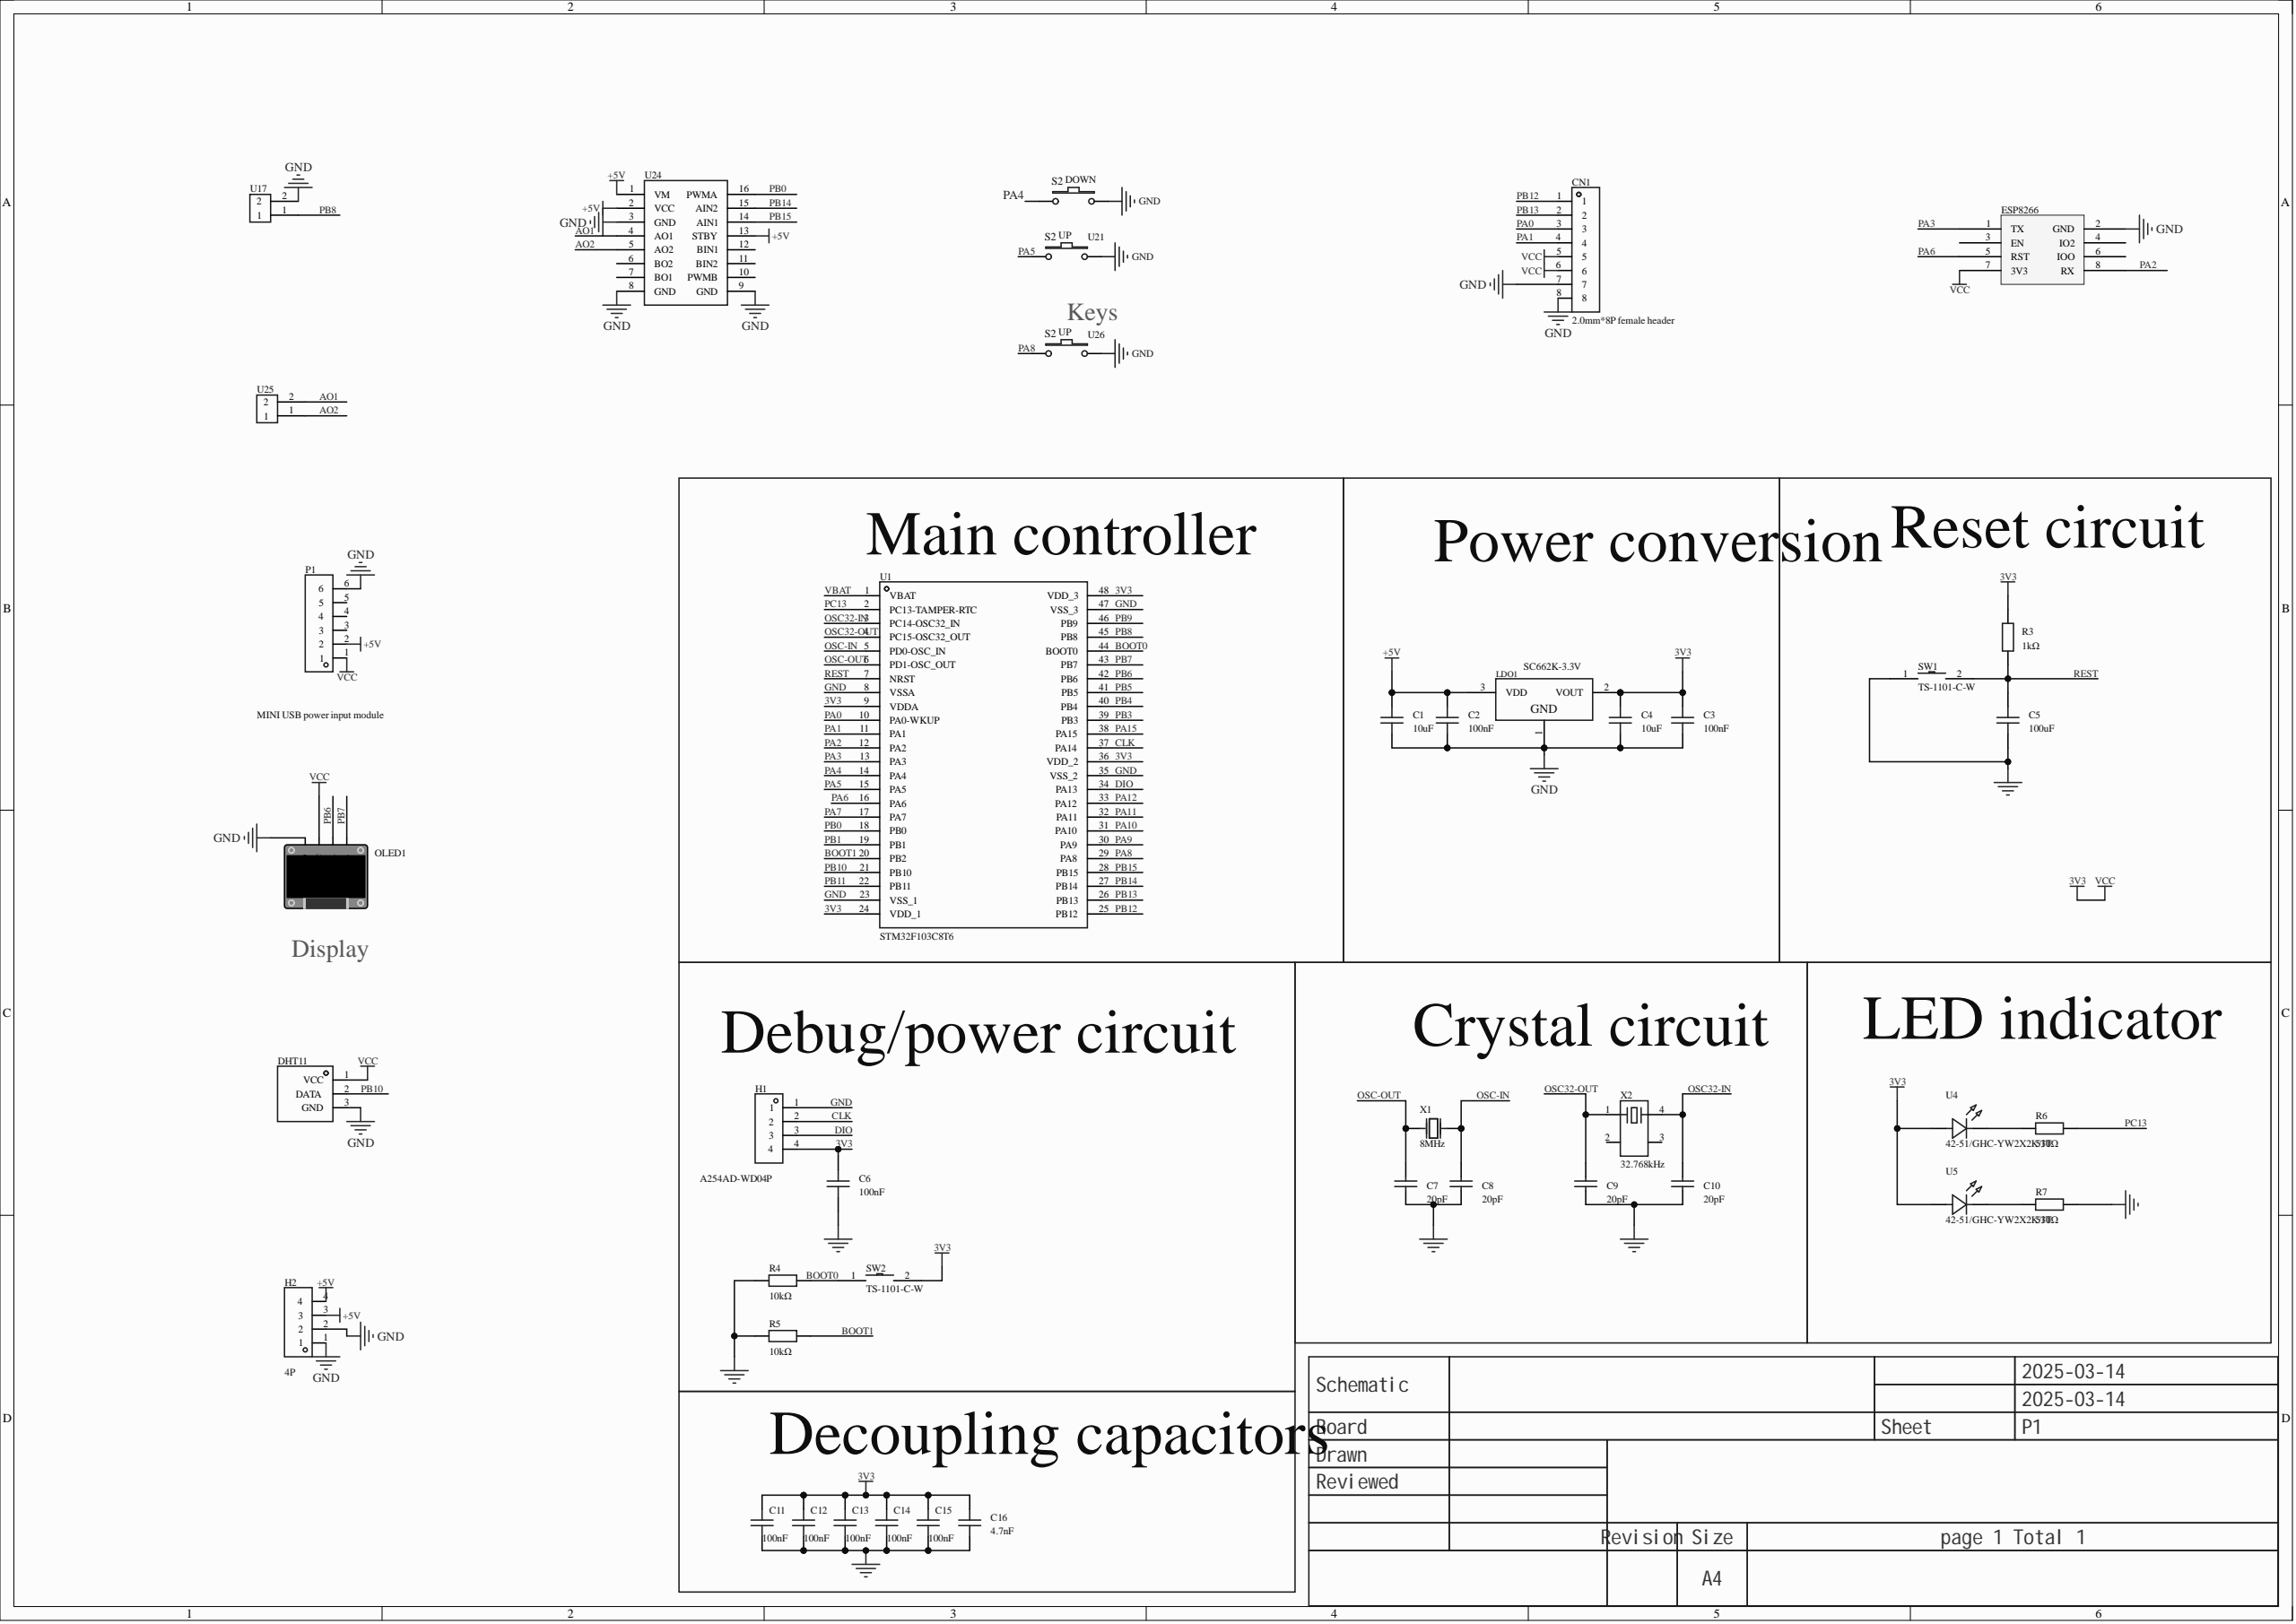Circuit board | Altium Designer | 42 parts | 34 nets
Bill of materials:
Comment,Description,Designator,Footprint,LibRef,Quantity
"10uF","Capacitance:10uF;Tolerance:±10%;Rated voltage:10V;Dielectric (temperature coefficient):X5R;","C1, C4","C0603","CL10A106KP8NNNC","2"
"100nF","Capacitance:100nF;Tolerance:±10%;Rated voltage:50V;Dielectric (temperature coefficient):X7R;","C2, C3, C6, C11, C12, C13, C14, C15","C0603","CC0603KRX7R9BB104, CGA0603X7R104K500JT","8"
"100uF","Capacitance:100uF;Tolerance:±20%;Rated voltage:10V;Dielectric (temperature coefficient):X5R;","C5","C1206","HGC1206R5107M100NSPJ","1"
"20pF","Capacitance:20pF;Tolerance:±5%;Rated voltage:50V;Dielectric (temperature coefficient):C0G;","C7, C8, C9, C10","C0603","CL10C200JB8NNNC","4"
"4.7nF","Capacitance:4.7nF;Tolerance:±10%;Rated voltage:50V;Dielectric (temperature coefficient):X7R;","C16","C0603","CGA0603X7R472K500JT","1"
"2.0mm*8P female header","","CN1","HDR-TH_8P-P1.27_2.0MM-8P","2.0mm*8P排母","1"
"","","DHT11","PIN3直插DHT11","DHT11","1"
"","","ESP8266","ESP8266-01S_Module","ESP8266-01S_Module*","1"
"A254AD-WD04P","插针结构:1x4P;间距:2.54mm;行距:-;圆针/方针:方针;安装类型:弯插;排数:单排;总PIN位数:4P;额定电流:3A;配合针长度:6mm;塑高:2.5mm;工作温度范围:-40℃~+105℃;","H1","HDR-TH_4P-P2.54-H-M-W10.2","A254AD-WD04P","1"
"4P","","H2","HDR-TH_4P-P2.54-V-M-3","4P排针","1"
"SC662K-3.3V","Output type:Fixed;Output polarity:Positive;Max input voltage:6V;Output voltage:3.3V;Output current:250mA;Power supply rejection ratio (PSRR):50dB@(1kHz);","LDO1","SOT-23-3_L2.9-W1.3-P1.90-LS2.4-BR","SC662K-3.3V","1"
"","","OLED1","0.96OLED_4P","0.96OLED模块_4P","1"
"MINI USB power input module","Socket structure:1x6P;Pitch:2.54mm;Row spacing:-;Mounting type:Through-hole;Rows:Single row;Total holes:6P;Plastic height:-;Contact material:-;Contact plating:-;","P1","HDR-TH_6P-P2.54-V-F","2.54-1*6P母","1"
"1kΩ","Resistor type:Thick film resistor;Resistance:1kΩ;Tolerance:±1%;Power:100mW;Max working voltage:75V;Temperature coefficient:±100ppm/?;","R3","R0603","RC0603FR-071KL","1"
"10kΩ","Resistor type:Thick film resistor;Resistance:10kΩ;Tolerance:±1%;Power:100mW;Max working voltage:75V;Temperature coefficient:±100ppm/?;","R4, R5","R0603","0603WAF1002T5E","2"
"510Ω","Resistor type:Thick film resistor;Resistance:510Ω;Tolerance:±1%;Power:100mW;Max working voltage:75V;Temperature coefficient:±100ppm/?;","R6, R7","R0603","0603WAF5100T5E","2"
"TS-1101-C-W","电路结构:单刀单掷;按钮形状:矩形按钮;作用力:260gf;安装方式:立贴;开关长度:6mm;开关宽度:3.6mm;开关高度:2.5mm;带支架:不带;触点电流:50mA;额定电压(AC):-;额定电压(DC):12V;额定功率:-;绝缘电阻:-;带灯:无;机械寿命:5万次;","SW1, SW2","SW-SMD_L6.0-W3.3-LS8.0","TS-1101-C-W","2"
"STM32F103C8T6","CPU内核:ARM-M3;程序存储容量:64KB;RAM总容量:20KB;GPIO端口数量:37;工作电压范围:2V~3.6V;CPU最大主频:72MHz;程序存储器类型:FLASH;","U1","LQFP-48_L7.0-W7.0-P0.50-LS9.0-BL","STM32F103C8T6","1"
"42-51/GHC-YW2X2K/3T","Emitted color:Emerald green;Forward current:-;Dominant wavelength:520nm~535nm;Luminous intensity:2850mcd;","U4, U5","LED-SMD_L1.6-W0.8-FD_GREEN-1","42-51/GHC-YW2X2K/3T","2"
"","","U17, U25","2p排针","2p排针","2"
"UP","","U21, U26","KEY-TH_4P复位按键","按键4P","2"
"DOWN","","U23","KEY-TH_4P复位按键","按键4P","1"
"","","U24","TB6612电机驱动","TB6612","1"
"8MHz","Crystal type:Through-hole crystal;Frequency:8MHz;Frequency tolerance (room temperature):±20ppm;Load capacitance:20pF;Frequency stability (full temperature):±30ppm;","X1","OSC-TH_L10.0-W4.5-P5.00","X49SD8MSD2SC","1"
"32.768kHz","Crystal type:SMD crystal;Frequency:32.768kHz;Frequency tolerance (room temperature):±20ppm;Load capacitance:12.5pF;","X2","MC-306_4P-L8.0-W3.2-P5.5-BL","Q13MC30610003","1"
Netlist (Protel format):
[
C1
C0603
10uF



]
[
C2
C0603
100nF



]
[
C3
C0603
100nF



]
[
C4
C0603
10uF



]
[
C5
C1206
100uF



]
[
C6
C0603
100nF



]
[
C7
C0603
20pF



]
[
C8
C0603
20pF



]
[
C9
C0603
20pF



]
[
C10
C0603
20pF



]
[
C11
C0603
100nF



]
[
C12
C0603
100nF



]
[
C13
C0603
100nF



]
[
C14
C0603
100nF



]
[
C15
C0603
100nF



]
[
C16
C0603
4.7nF



]
[
CN1
HDR-TH_8P-P1.27_2.0MM-8P
2.0mm*8P female header



]
[
DHT11
PIN3直插DHT11




]
[
ESP8266
ESP8266-01S_Module




]
[
H1
HDR-TH_4P-P2.54-H-M-W10.2
A254AD-WD04P



]
[
H2
HDR-TH_4P-P2.54-V-M-3
4P



]
[
LDO1
SOT-23-3_L2.9-W1.3-P1.90-LS2.4-BR
SC662K-3.3V



]
[
OLED1
0.96OLED_4P




]
[
P1
HDR-TH_6P-P2.54-V-F
MINI USB power input module



]
[
R3
R0603
1kΩ



]
[
R4
R0603
10kΩ



]
[
R5
R0603
10kΩ



]
[
R6
R0603
510Ω



]
[
R7
R0603
510Ω



]
[
SW1
SW-SMD_L6.0-W3.3-LS8.0
TS-1101-C-W



]
[
SW2
SW-SMD_L6.0-W3.3-LS8.0
TS-1101-C-W



]
[
U1
LQFP-48_L7.0-W7.0-P0.50-LS9.0-BL
STM32F103C8T6



]
[
U4
LED-SMD_L1.6-W0.8-FD_GREEN-1
42-51/GHC-YW2X2K/3T



]
[
U5
LED-SMD_L1.6-W0.8-FD_GREEN-1
42-51/GHC-YW2X2K/3T



]
[
U17
2p排针




]
[
U21
KEY-TH_4P复位按键
UP



]
[
U23
KEY-TH_4P复位按键
DOWN



]
[
U24
TB6612电机驱动




]
[
U25
2p排针




]
[
U26
KEY-TH_4P复位按键
UP



]
[
X1
OSC-TH_L10.0-W4.5-P5.00
8MHz



]
[
X2
MC-306_4P-L8.0-W3.2-P5.5-BL
32.768kHz



]
(
REST
C5-2
R3-1
SW1-2
U1-7
)
(
PC13
R6-2
U1-2
)
(
PB15
U1-28
U24-14
)
(
PB14
U1-27
U24-15
)
(
PB13
CN1-2
U1-26
)
(
PB12
CN1-1
U1-25
)
(
PB10
DHT11-2
U1-21
)
(
PB8
U1-45
U17-1
)
(
PB7
OLED1-4
U1-43
)
(
PB6
OLED1-3
U1-42
)
(
PB0
U1-18
U24-16
)
(
PA8
U1-29
U26-1
)
(
PA6
ESP8266-5
U1-16
)
(
PA5
U1-15
U21-1
)
(
PA4
U1-14
U23-1
)
(
PA3
ESP8266-1
U1-13
)
(
PA2
ESP8266-8
U1-12
)
(
PA1
CN1-4
U1-11
)
(
PA0
CN1-3
U1-10
)
(
OSC-OUT
C7-2
U1-6
X1-2
)
(
OSC-IN
C8-2
U1-5
X1-1
)
(
OSC32-OUT
C9-2
U1-4
X2-1
)
(
OSC32-IN
C10-2
U1-3
X2-4
)
(
NetR7_1
R7-1
U5-2
)
(
NetR6_1
R6-1
U4-2
)
(
GND
C1-1
C2-1
C3-1
C4-1
C5-1
C6-1
C7-1
C8-1
C9-1
C10-1
C11-1
C12-1
C13-1
C14-1
C15-1
C16-1
CN1-7
CN1-8
DHT11-3
ESP8266-2
H1-1
H2-1
H2-2
LDO1-1
OLED1-1
P1-6
R4-1
R5-1
R7-2
SW1-1
U1-8
U1-23
U1-35
U1-47
U17-2
U21-3
U23-3
U24-3
U24-8
U24-9
U26-3
)
(
DIO
H1-3
U1-34
)
(
CLK
H1-2
U1-37
)
(
BOOT1
R5-2
U1-20
)
(
BOOT0
R4-2
SW2-1
U1-44
)
(
AO2
U24-5
U25-1
)
(
AO1
U24-4
U25-2
)
(
+5V
C1-2
C2-2
H2-3
H2-4
LDO1-3
P1-2
U24-1
U24-2
U24-13
)
(
3V3
C3-2
C4-2
C6-2
C11-2
C12-2
C13-2
C14-2
C15-2
C16-2
CN1-5
CN1-6
DHT11-1
ESP8266-7
H1-4
LDO1-2
OLED1-2
P1-1
R3-2
SW2-2
U1-9
U1-24
U1-36
U1-48
U4-1
U5-1
)